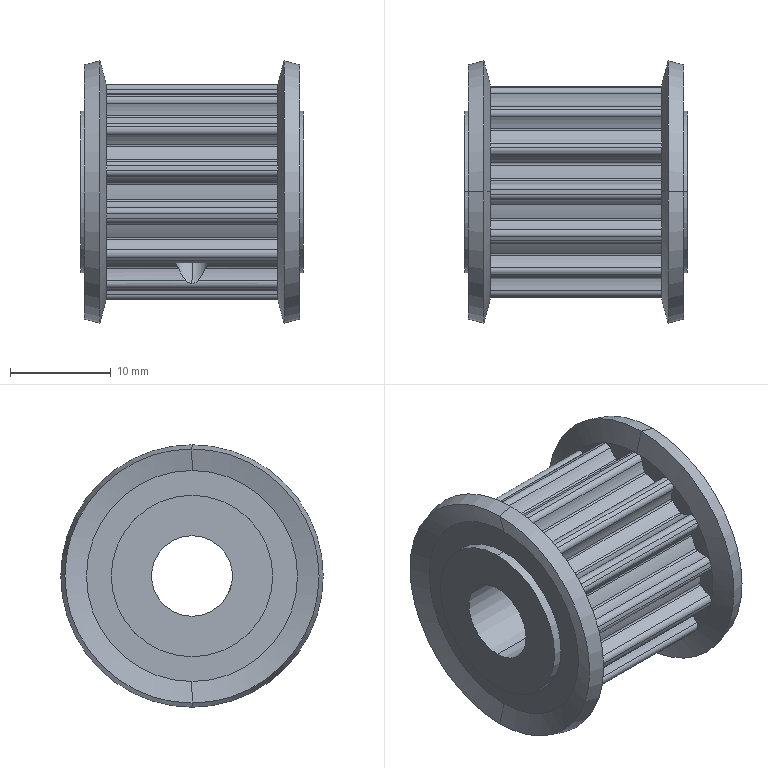Part | SolidWorks | features BaseBody 1 | 1 solid | 177 faces | box 22 x 26 x 26 mm | volume 5766 mm3 | cylinder 133 | plane 32 | cone 12 | commonest cylinder face diameters 0.5 x32 6.55 x32 1.1 x28 17.78 x16 21.32 x15 3.242 x4